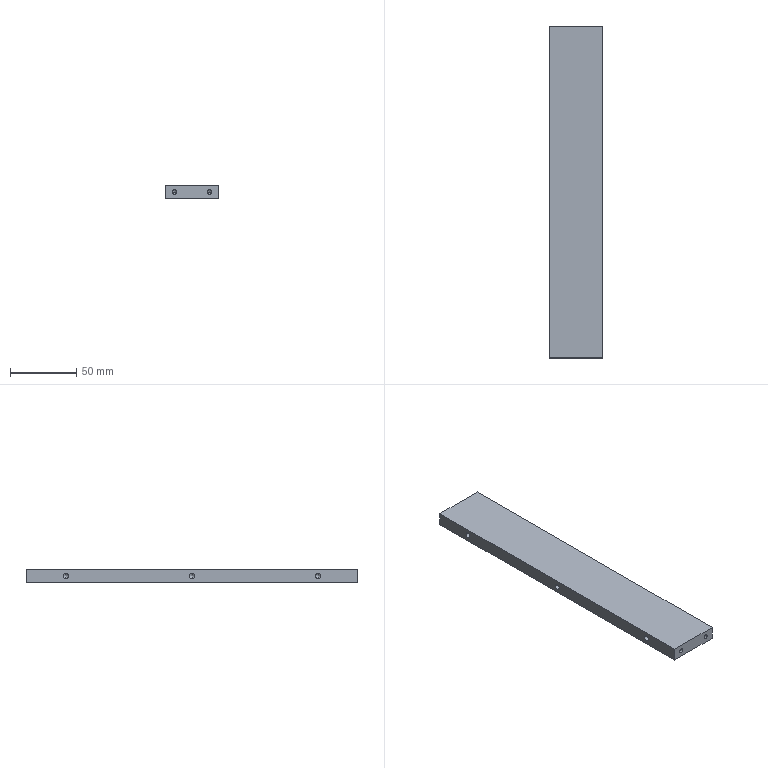Part | SolidWorks | features BaseBody 1 | 1 solid | 34 faces | box 40 x 250 x 10 mm | volume 99178 mm3 | cylinder 14 | cone 14 | plane 6 | commonest cylinder face diameters 4.134 x6 2.487 x4 3.242 x4
STEP:
#1=CARTESIAN_POINT('',(-243.627,247.034,3.757));
#2=VERTEX_POINT('',#1);
#3=CARTESIAN_POINT('',(-243.627,247.034,6.243));
#4=VERTEX_POINT('',#3);
#5=CARTESIAN_POINT('',(-243.627,247.034,5.));
#6=DIRECTION('',(0.,1.,0.));
#7=DIRECTION('',(0.,0.,1.));
#8=AXIS2_PLACEMENT_3D('',#5,#6,#7);
#9=CIRCLE('',#8,1.243);
#10=EDGE_CURVE('',#2,#4,#9,.T.);
#11=ORIENTED_EDGE('',*,*,#10,.F.);
#12=CARTESIAN_POINT('',(-243.627,259.034,3.757));
#13=VERTEX_POINT('',#12);
#14=CARTESIAN_POINT('',(-243.627,253.034,3.757));
#15=DIRECTION('',(0.,1.,0.));
#16=VECTOR('',#15,1000.);
#17=LINE('',#14,#16);
#18=EDGE_CURVE('',#2,#13,#17,.T.);
#19=ORIENTED_EDGE('',*,*,#18,.T.);
#20=CARTESIAN_POINT('',(-243.627,259.034,6.244));
#21=VERTEX_POINT('',#20);
#22=CARTESIAN_POINT('',(-243.627,259.034,5.));
#23=DIRECTION('',(0.,-1.,0.));
#24=DIRECTION('',(0.,0.,1.));
#25=AXIS2_PLACEMENT_3D('',#22,#23,#24);
#26=CIRCLE('',#25,1.243);
#27=EDGE_CURVE('',#21,#13,#26,.T.);
#28=ORIENTED_EDGE('',*,*,#27,.F.);
#29=CARTESIAN_POINT('',(-243.627,253.034,6.244));
#30=DIRECTION('',(0.,1.,0.));
#31=VECTOR('',#30,1000.);
#32=LINE('',#29,#31);
#33=EDGE_CURVE('',#4,#21,#32,.T.);
#34=ORIENTED_EDGE('',*,*,#33,.F.);
#35=EDGE_LOOP('',(#11,#19,#28,#34));
#36=FACE_OUTER_BOUND('',#35,.T.);
#37=CARTESIAN_POINT('',(-243.627,253.034,5.));
#38=DIRECTION('',(0.,1.,0.));
#39=DIRECTION('',(0.,0.,1.));
#40=AXIS2_PLACEMENT_3D('',#37,#38,#39);
#41=CYLINDRICAL_SURFACE('',#40,1.243);
#42=ADVANCED_FACE('',(#36),#41,.F.);
#43=CARTESIAN_POINT('',(-217.627,247.034,3.757));
#44=VERTEX_POINT('',#43);
#45=CARTESIAN_POINT('',(-217.627,247.034,6.243));
#46=VERTEX_POINT('',#45);
#47=CARTESIAN_POINT('',(-217.627,247.034,5.));
#48=DIRECTION('',(0.,1.,0.));
#49=DIRECTION('',(0.,0.,1.));
#50=AXIS2_PLACEMENT_3D('',#47,#48,#49);
#51=CIRCLE('',#50,1.243);
#52=EDGE_CURVE('',#44,#46,#51,.T.);
#53=ORIENTED_EDGE('',*,*,#52,.F.);
#54=CARTESIAN_POINT('',(-217.627,259.034,3.757));
#55=VERTEX_POINT('',#54);
#56=CARTESIAN_POINT('',(-217.627,253.034,3.757));
#57=DIRECTION('',(0.,1.,0.));
#58=VECTOR('',#57,1000.);
#59=LINE('',#56,#58);
#60=EDGE_CURVE('',#44,#55,#59,.T.);
#61=ORIENTED_EDGE('',*,*,#60,.T.);
#62=CARTESIAN_POINT('',(-217.627,259.034,6.244));
#63=VERTEX_POINT('',#62);
#64=CARTESIAN_POINT('',(-217.627,259.034,5.));
#65=DIRECTION('',(0.,-1.,0.));
#66=DIRECTION('',(0.,0.,1.));
#67=AXIS2_PLACEMENT_3D('',#64,#65,#66);
#68=CIRCLE('',#67,1.243);
#69=EDGE_CURVE('',#63,#55,#68,.T.);
#70=ORIENTED_EDGE('',*,*,#69,.F.);
#71=CARTESIAN_POINT('',(-217.627,253.034,6.244));
#72=DIRECTION('',(0.,1.,0.));
#73=VECTOR('',#72,1000.);
#74=LINE('',#71,#73);
#75=EDGE_CURVE('',#46,#63,#74,.T.);
#76=ORIENTED_EDGE('',*,*,#75,.F.);
#77=EDGE_LOOP('',(#53,#61,#70,#76));
#78=FACE_OUTER_BOUND('',#77,.T.);
#79=CARTESIAN_POINT('',(-217.627,253.034,5.));
#80=DIRECTION('',(0.,1.,0.));
#81=DIRECTION('',(0.,0.,1.));
#82=AXIS2_PLACEMENT_3D('',#79,#80,#81);
#83=CYLINDRICAL_SURFACE('',#82,1.243);
#84=ADVANCED_FACE('',(#78),#83,.F.);
#85=CARTESIAN_POINT('',(-245.248,21.034,5.));
#86=VERTEX_POINT('',#85);
#87=CARTESIAN_POINT('',(-242.006,21.034,5.));
#88=VERTEX_POINT('',#87);
#89=CARTESIAN_POINT('',(-243.627,21.034,5.));
#90=DIRECTION('',(0.,-1.,0.));
#91=DIRECTION('',(1.,0.,0.));
#92=AXIS2_PLACEMENT_3D('',#89,#90,#91);
#93=CIRCLE('',#92,1.621);
#94=EDGE_CURVE('',#86,#88,#93,.T.);
#95=ORIENTED_EDGE('',*,*,#94,.F.);
#96=CARTESIAN_POINT('',(-245.248,9.034,5.));
#97=VERTEX_POINT('',#96);
#98=CARTESIAN_POINT('',(-245.248,15.034,5.));
#99=DIRECTION('',(0.,-1.,0.));
#100=VECTOR('',#99,1000.);
#101=LINE('',#98,#100);
#102=EDGE_CURVE('',#86,#97,#101,.T.);
#103=ORIENTED_EDGE('',*,*,#102,.T.);
#104=CARTESIAN_POINT('',(-242.006,9.034,5.));
#105=VERTEX_POINT('',#104);
#106=CARTESIAN_POINT('',(-243.627,9.034,5.));
#107=DIRECTION('',(0.,1.,0.));
#108=DIRECTION('',(1.,0.,0.));
#109=AXIS2_PLACEMENT_3D('',#106,#107,#108);
#110=CIRCLE('',#109,1.621);
#111=EDGE_CURVE('',#105,#97,#110,.T.);
#112=ORIENTED_EDGE('',*,*,#111,.F.);
#113=CARTESIAN_POINT('',(-242.006,15.034,5.));
#114=DIRECTION('',(0.,-1.,0.));
#115=VECTOR('',#114,1000.);
#116=LINE('',#113,#115);
#117=EDGE_CURVE('',#88,#105,#116,.T.);
#118=ORIENTED_EDGE('',*,*,#117,.F.);
#119=EDGE_LOOP('',(#95,#103,#112,#118));
#120=FACE_OUTER_BOUND('',#119,.T.);
#121=CARTESIAN_POINT('',(-243.627,15.034,5.));
#122=DIRECTION('',(0.,-1.,0.));
#123=DIRECTION('',(1.,0.,0.));
#124=AXIS2_PLACEMENT_3D('',#121,#122,#123);
#125=CYLINDRICAL_SURFACE('',#124,1.621);
#126=ADVANCED_FACE('',(#120),#125,.F.);
#127=CARTESIAN_POINT('',(-219.248,21.034,5.));
#128=VERTEX_POINT('',#127);
#129=CARTESIAN_POINT('',(-216.006,21.034,5.));
#130=VERTEX_POINT('',#129);
#131=CARTESIAN_POINT('',(-217.627,21.034,5.));
#132=DIRECTION('',(0.,-1.,0.));
#133=DIRECTION('',(1.,0.,0.));
#134=AXIS2_PLACEMENT_3D('',#131,#132,#133);
#135=CIRCLE('',#134,1.621);
#136=EDGE_CURVE('',#128,#130,#135,.T.);
#137=ORIENTED_EDGE('',*,*,#136,.F.);
#138=CARTESIAN_POINT('',(-219.248,9.034,5.));
#139=VERTEX_POINT('',#138);
#140=CARTESIAN_POINT('',(-219.248,15.034,5.));
#141=DIRECTION('',(0.,-1.,0.));
#142=VECTOR('',#141,1000.);
#143=LINE('',#140,#142);
#144=EDGE_CURVE('',#128,#139,#143,.T.);
#145=ORIENTED_EDGE('',*,*,#144,.T.);
#146=CARTESIAN_POINT('',(-216.006,9.034,5.));
#147=VERTEX_POINT('',#146);
#148=CARTESIAN_POINT('',(-217.627,9.034,5.));
#149=DIRECTION('',(0.,1.,0.));
#150=DIRECTION('',(1.,0.,0.));
#151=AXIS2_PLACEMENT_3D('',#148,#149,#150);
#152=CIRCLE('',#151,1.621);
#153=EDGE_CURVE('',#147,#139,#152,.T.);
#154=ORIENTED_EDGE('',*,*,#153,.F.);
#155=CARTESIAN_POINT('',(-216.006,15.034,5.));
#156=DIRECTION('',(0.,-1.,0.));
#157=VECTOR('',#156,1000.);
#158=LINE('',#155,#157);
#159=EDGE_CURVE('',#130,#147,#158,.T.);
#160=ORIENTED_EDGE('',*,*,#159,.F.);
#161=EDGE_LOOP('',(#137,#145,#154,#160));
#162=FACE_OUTER_BOUND('',#161,.T.);
#163=CARTESIAN_POINT('',(-217.627,15.034,5.));
#164=DIRECTION('',(0.,-1.,0.));
#165=DIRECTION('',(1.,0.,0.));
#166=AXIS2_PLACEMENT_3D('',#163,#164,#165);
#167=CYLINDRICAL_SURFACE('',#166,1.621);
#168=ADVANCED_FACE('',(#162),#167,.F.);
#169=CARTESIAN_POINT('',(-238.627,231.101,5.));
#170=VERTEX_POINT('',#169);
#171=CARTESIAN_POINT('',(-238.627,229.034,2.933));
#172=VERTEX_POINT('',#171);
#173=CARTESIAN_POINT('',(-238.627,229.034,5.));
#174=DIRECTION('',(-1.,0.,0.));
#175=DIRECTION('',(0.,-1.,0.));
#176=AXIS2_PLACEMENT_3D('',#173,#174,#175);
#177=CIRCLE('',#176,2.067);
#178=EDGE_CURVE('',#170,#172,#177,.T.);
#179=ORIENTED_EDGE('',*,*,#178,.F.);
#180=CARTESIAN_POINT('',(-250.627,231.101,5.));
#181=VERTEX_POINT('',#180);
#182=CARTESIAN_POINT('',(-244.627,231.101,5.));
#183=DIRECTION('',(-1.,0.,0.));
#184=VECTOR('',#183,1000.);
#185=LINE('',#182,#184);
#186=EDGE_CURVE('',#170,#181,#185,.T.);
#187=ORIENTED_EDGE('',*,*,#186,.T.);
#188=CARTESIAN_POINT('',(-250.627,226.967,5.));
#189=VERTEX_POINT('',#188);
#190=CARTESIAN_POINT('',(-250.627,229.034,5.));
#191=DIRECTION('',(1.,0.,0.));
#192=DIRECTION('',(0.,-1.,0.));
#193=AXIS2_PLACEMENT_3D('',#190,#191,#192);
#194=CIRCLE('',#193,2.067);
#195=EDGE_CURVE('',#189,#181,#194,.T.);
#196=ORIENTED_EDGE('',*,*,#195,.F.);
#197=CARTESIAN_POINT('',(-238.627,226.967,5.));
#198=VERTEX_POINT('',#197);
#199=CARTESIAN_POINT('',(-244.627,226.967,5.));
#200=DIRECTION('',(-1.,0.,0.));
#201=VECTOR('',#200,1000.);
#202=LINE('',#199,#201);
#203=EDGE_CURVE('',#198,#189,#202,.T.);
#204=ORIENTED_EDGE('',*,*,#203,.F.);
#205=CARTESIAN_POINT('',(-238.627,229.034,5.));
#206=DIRECTION('',(-1.,0.,0.));
#207=DIRECTION('',(0.,-1.,0.));
#208=AXIS2_PLACEMENT_3D('',#205,#206,#207);
#209=CIRCLE('',#208,2.067);
#210=EDGE_CURVE('',#172,#198,#209,.T.);
#211=ORIENTED_EDGE('',*,*,#210,.F.);
#212=EDGE_LOOP('',(#179,#187,#196,#204,#211));
#213=FACE_OUTER_BOUND('',#212,.T.);
#214=CARTESIAN_POINT('',(-244.627,229.034,5.));
#215=DIRECTION('',(-1.,0.,0.));
#216=DIRECTION('',(0.,-1.,0.));
#217=AXIS2_PLACEMENT_3D('',#214,#215,#216);
#218=CYLINDRICAL_SURFACE('',#217,2.067);
#219=ADVANCED_FACE('',(#213),#218,.F.);
#220=CARTESIAN_POINT('',(-238.627,136.101,5.));
#221=VERTEX_POINT('',#220);
#222=CARTESIAN_POINT('',(-238.627,134.034,2.933));
#223=VERTEX_POINT('',#222);
#224=CARTESIAN_POINT('',(-238.627,134.034,5.));
#225=DIRECTION('',(-1.,0.,0.));
#226=DIRECTION('',(0.,-1.,0.));
#227=AXIS2_PLACEMENT_3D('',#224,#225,#226);
#228=CIRCLE('',#227,2.067);
#229=EDGE_CURVE('',#221,#223,#228,.T.);
#230=ORIENTED_EDGE('',*,*,#229,.F.);
#231=CARTESIAN_POINT('',(-250.627,136.101,5.));
#232=VERTEX_POINT('',#231);
#233=CARTESIAN_POINT('',(-244.627,136.101,5.));
#234=DIRECTION('',(-1.,0.,0.));
#235=VECTOR('',#234,1000.);
#236=LINE('',#233,#235);
#237=EDGE_CURVE('',#221,#232,#236,.T.);
#238=ORIENTED_EDGE('',*,*,#237,.T.);
#239=CARTESIAN_POINT('',(-250.627,131.967,5.));
#240=VERTEX_POINT('',#239);
#241=CARTESIAN_POINT('',(-250.627,134.034,5.));
#242=DIRECTION('',(1.,0.,0.));
#243=DIRECTION('',(0.,-1.,0.));
#244=AXIS2_PLACEMENT_3D('',#241,#242,#243);
#245=CIRCLE('',#244,2.067);
#246=EDGE_CURVE('',#240,#232,#245,.T.);
#247=ORIENTED_EDGE('',*,*,#246,.F.);
#248=CARTESIAN_POINT('',(-238.627,131.967,5.));
#249=VERTEX_POINT('',#248);
#250=CARTESIAN_POINT('',(-244.627,131.967,5.));
#251=DIRECTION('',(-1.,0.,0.));
#252=VECTOR('',#251,1000.);
#253=LINE('',#250,#252);
#254=EDGE_CURVE('',#249,#240,#253,.T.);
#255=ORIENTED_EDGE('',*,*,#254,.F.);
#256=CARTESIAN_POINT('',(-238.627,134.034,5.));
#257=DIRECTION('',(-1.,0.,0.));
#258=DIRECTION('',(0.,-1.,0.));
#259=AXIS2_PLACEMENT_3D('',#256,#257,#258);
#260=CIRCLE('',#259,2.067);
#261=EDGE_CURVE('',#223,#249,#260,.T.);
#262=ORIENTED_EDGE('',*,*,#261,.F.);
#263=EDGE_LOOP('',(#230,#238,#247,#255,#262));
#264=FACE_OUTER_BOUND('',#263,.T.);
#265=CARTESIAN_POINT('',(-244.627,134.034,5.));
#266=DIRECTION('',(-1.,0.,0.));
#267=DIRECTION('',(0.,-1.,0.));
#268=AXIS2_PLACEMENT_3D('',#265,#266,#267);
#269=CYLINDRICAL_SURFACE('',#268,2.067);
#270=ADVANCED_FACE('',(#264),#269,.F.);
#271=CARTESIAN_POINT('',(-238.627,41.101,5.));
#272=VERTEX_POINT('',#271);
#273=CARTESIAN_POINT('',(-238.627,39.034,2.933));
#274=VERTEX_POINT('',#273);
#275=CARTESIAN_POINT('',(-238.627,39.034,5.));
#276=DIRECTION('',(-1.,0.,0.));
#277=DIRECTION('',(0.,-1.,0.));
#278=AXIS2_PLACEMENT_3D('',#275,#276,#277);
#279=CIRCLE('',#278,2.067);
#280=EDGE_CURVE('',#272,#274,#279,.T.);
#281=ORIENTED_EDGE('',*,*,#280,.F.);
#282=CARTESIAN_POINT('',(-250.627,41.101,5.));
#283=VERTEX_POINT('',#282);
#284=CARTESIAN_POINT('',(-244.627,41.101,5.));
#285=DIRECTION('',(-1.,0.,0.));
#286=VECTOR('',#285,1000.);
#287=LINE('',#284,#286);
#288=EDGE_CURVE('',#272,#283,#287,.T.);
#289=ORIENTED_EDGE('',*,*,#288,.T.);
#290=CARTESIAN_POINT('',(-250.627,36.967,5.));
#291=VERTEX_POINT('',#290);
#292=CARTESIAN_POINT('',(-250.627,39.034,5.));
#293=DIRECTION('',(1.,0.,0.));
#294=DIRECTION('',(0.,-1.,0.));
#295=AXIS2_PLACEMENT_3D('',#292,#293,#294);
#296=CIRCLE('',#295,2.067);
#297=EDGE_CURVE('',#291,#283,#296,.T.);
#298=ORIENTED_EDGE('',*,*,#297,.F.);
#299=CARTESIAN_POINT('',(-238.627,36.967,5.));
#300=VERTEX_POINT('',#299);
#301=CARTESIAN_POINT('',(-244.627,36.967,5.));
#302=DIRECTION('',(-1.,0.,0.));
#303=VECTOR('',#302,1000.);
#304=LINE('',#301,#303);
#305=EDGE_CURVE('',#300,#291,#304,.T.);
#306=ORIENTED_EDGE('',*,*,#305,.F.);
#307=CARTESIAN_POINT('',(-238.627,39.034,5.));
#308=DIRECTION('',(-1.,0.,0.));
#309=DIRECTION('',(0.,-1.,0.));
#310=AXIS2_PLACEMENT_3D('',#307,#308,#309);
#311=CIRCLE('',#310,2.067);
#312=EDGE_CURVE('',#274,#300,#311,.T.);
#313=ORIENTED_EDGE('',*,*,#312,.F.);
#314=EDGE_LOOP('',(#281,#289,#298,#306,#313));
#315=FACE_OUTER_BOUND('',#314,.T.);
#316=CARTESIAN_POINT('',(-244.627,39.034,5.));
#317=DIRECTION('',(-1.,0.,0.));
#318=DIRECTION('',(0.,-1.,0.));
#319=AXIS2_PLACEMENT_3D('',#316,#317,#318);
#320=CYLINDRICAL_SURFACE('',#319,2.067);
#321=ADVANCED_FACE('',(#315),#320,.F.);
#322=CARTESIAN_POINT('',(-243.627,246.287,5.));
#323=VERTEX_POINT('',#322);
#324=CARTESIAN_POINT('',(-243.627,247.034,6.243));
#325=DIRECTION('',(0.,0.515,0.8572));
#326=VECTOR('',#325,1000.);
#327=LINE('',#324,#326);
#328=EDGE_CURVE('',#323,#4,#327,.T.);
#329=ORIENTED_EDGE('',*,*,#328,.F.);
#330=CARTESIAN_POINT('',(-243.627,247.034,3.757));
#331=DIRECTION('',(0.,0.515,-0.8572));
#332=VECTOR('',#331,1000.);
#333=LINE('',#330,#332);
#334=EDGE_CURVE('',#323,#2,#333,.T.);
#335=ORIENTED_EDGE('',*,*,#334,.T.);
#336=ORIENTED_EDGE('',*,*,#10,.T.);
#337=EDGE_LOOP('',(#329,#335,#336));
#338=FACE_OUTER_BOUND('',#337,.T.);
#339=CARTESIAN_POINT('',(-243.627,247.034,5.));
#340=DIRECTION('',(0.,1.,0.));
#341=DIRECTION('',(0.,0.,1.));
#342=AXIS2_PLACEMENT_3D('',#339,#340,#341);
#343=CONICAL_SURFACE('',#342,1.243,1.03);
#344=ADVANCED_FACE('',(#338),#343,.F.);
#345=CARTESIAN_POINT('',(-217.627,246.287,5.));
#346=VERTEX_POINT('',#345);
#347=CARTESIAN_POINT('',(-217.627,247.034,6.243));
#348=DIRECTION('',(0.,0.515,0.8572));
#349=VECTOR('',#348,1000.);
#350=LINE('',#347,#349);
#351=EDGE_CURVE('',#346,#46,#350,.T.);
#352=ORIENTED_EDGE('',*,*,#351,.F.);
#353=CARTESIAN_POINT('',(-217.627,247.034,3.757));
#354=DIRECTION('',(0.,0.515,-0.8572));
#355=VECTOR('',#354,1000.);
#356=LINE('',#353,#355);
#357=EDGE_CURVE('',#346,#44,#356,.T.);
#358=ORIENTED_EDGE('',*,*,#357,.T.);
#359=ORIENTED_EDGE('',*,*,#52,.T.);
#360=EDGE_LOOP('',(#352,#358,#359));
#361=FACE_OUTER_BOUND('',#360,.T.);
#362=CARTESIAN_POINT('',(-217.627,247.034,5.));
#363=DIRECTION('',(0.,1.,0.));
#364=DIRECTION('',(0.,0.,1.));
#365=AXIS2_PLACEMENT_3D('',#362,#363,#364);
#366=CONICAL_SURFACE('',#365,1.243,1.03);
#367=ADVANCED_FACE('',(#361),#366,.F.);
#368=CARTESIAN_POINT('',(-243.627,22.008,5.));
#369=VERTEX_POINT('',#368);
#370=CARTESIAN_POINT('',(-242.006,21.034,5.));
#371=DIRECTION('',(0.8572,-0.515,0.));
#372=VECTOR('',#371,1000.);
#373=LINE('',#370,#372);
#374=EDGE_CURVE('',#369,#88,#373,.T.);
#375=ORIENTED_EDGE('',*,*,#374,.F.);
#376=CARTESIAN_POINT('',(-245.248,21.034,5.));
#377=DIRECTION('',(-0.8572,-0.515,0.));
#378=VECTOR('',#377,1000.);
#379=LINE('',#376,#378);
#380=EDGE_CURVE('',#369,#86,#379,.T.);
#381=ORIENTED_EDGE('',*,*,#380,.T.);
#382=ORIENTED_EDGE('',*,*,#94,.T.);
#383=EDGE_LOOP('',(#375,#381,#382));
#384=FACE_OUTER_BOUND('',#383,.T.);
#385=CARTESIAN_POINT('',(-243.627,21.034,5.));
#386=DIRECTION('',(0.,-1.,0.));
#387=DIRECTION('',(1.,0.,0.));
#388=AXIS2_PLACEMENT_3D('',#385,#386,#387);
#389=CONICAL_SURFACE('',#388,1.621,1.03);
#390=ADVANCED_FACE('',(#384),#389,.F.);
#391=CARTESIAN_POINT('',(-217.627,22.008,5.));
#392=VERTEX_POINT('',#391);
#393=CARTESIAN_POINT('',(-216.006,21.034,5.));
#394=DIRECTION('',(0.8572,-0.515,0.));
#395=VECTOR('',#394,1000.);
#396=LINE('',#393,#395);
#397=EDGE_CURVE('',#392,#130,#396,.T.);
#398=ORIENTED_EDGE('',*,*,#397,.F.);
#399=CARTESIAN_POINT('',(-219.248,21.034,5.));
#400=DIRECTION('',(-0.8572,-0.515,0.));
#401=VECTOR('',#400,1000.);
#402=LINE('',#399,#401);
#403=EDGE_CURVE('',#392,#128,#402,.T.);
#404=ORIENTED_EDGE('',*,*,#403,.T.);
#405=ORIENTED_EDGE('',*,*,#136,.T.);
#406=EDGE_LOOP('',(#398,#404,#405));
#407=FACE_OUTER_BOUND('',#406,.T.);
#408=CARTESIAN_POINT('',(-217.627,21.034,5.));
#409=DIRECTION('',(0.,-1.,0.));
#410=DIRECTION('',(1.,0.,0.));
#411=AXIS2_PLACEMENT_3D('',#408,#409,#410);
#412=CONICAL_SURFACE('',#411,1.621,1.03);
#413=ADVANCED_FACE('',(#407),#412,.F.);
#414=CARTESIAN_POINT('',(-237.385,229.034,5.));
#415=VERTEX_POINT('',#414);
#416=CARTESIAN_POINT('',(-238.627,229.034,7.067));
#417=VERTEX_POINT('',#416);
#418=CARTESIAN_POINT('',(-238.627,229.034,7.067));
#419=DIRECTION('',(-0.515,0.,0.8572));
#420=VECTOR('',#419,1000.);
#421=LINE('',#418,#420);
#422=EDGE_CURVE('',#415,#417,#421,.T.);
#423=ORIENTED_EDGE('',*,*,#422,.F.);
#424=CARTESIAN_POINT('',(-238.627,229.034,2.933));
#425=DIRECTION('',(-0.515,0.,-0.8572));
#426=VECTOR('',#425,1000.);
#427=LINE('',#424,#426);
#428=EDGE_CURVE('',#415,#172,#427,.T.);
#429=ORIENTED_EDGE('',*,*,#428,.T.);
#430=ORIENTED_EDGE('',*,*,#210,.T.);
#431=CARTESIAN_POINT('',(-238.627,229.034,5.));
#432=DIRECTION('',(-1.,0.,0.));
#433=DIRECTION('',(0.,-1.,0.));
#434=AXIS2_PLACEMENT_3D('',#431,#432,#433);
#435=CIRCLE('',#434,2.067);
#436=EDGE_CURVE('',#198,#417,#435,.T.);
#437=ORIENTED_EDGE('',*,*,#436,.T.);
#438=EDGE_LOOP('',(#423,#429,#430,#437));
#439=FACE_OUTER_BOUND('',#438,.T.);
#440=CARTESIAN_POINT('',(-238.627,229.034,5.));
#441=DIRECTION('',(-1.,0.,0.));
#442=DIRECTION('',(0.,0.,1.));
#443=AXIS2_PLACEMENT_3D('',#440,#441,#442);
#444=CONICAL_SURFACE('',#443,2.067,1.03);
#445=ADVANCED_FACE('',(#439),#444,.F.);
#446=CARTESIAN_POINT('',(-237.385,134.034,5.));
#447=VERTEX_POINT('',#446);
#448=CARTESIAN_POINT('',(-238.627,134.034,7.067));
#449=VERTEX_POINT('',#448);
#450=CARTESIAN_POINT('',(-238.627,134.034,7.067));
#451=DIRECTION('',(-0.515,0.,0.8572));
#452=VECTOR('',#451,1000.);
#453=LINE('',#450,#452);
#454=EDGE_CURVE('',#447,#449,#453,.T.);
#455=ORIENTED_EDGE('',*,*,#454,.F.);
#456=CARTESIAN_POINT('',(-238.627,134.034,2.933));
#457=DIRECTION('',(-0.515,0.,-0.8572));
#458=VECTOR('',#457,1000.);
#459=LINE('',#456,#458);
#460=EDGE_CURVE('',#447,#223,#459,.T.);
#461=ORIENTED_EDGE('',*,*,#460,.T.);
#462=ORIENTED_EDGE('',*,*,#261,.T.);
#463=CARTESIAN_POINT('',(-238.627,134.034,5.));
#464=DIRECTION('',(-1.,0.,0.));
#465=DIRECTION('',(0.,-1.,0.));
#466=AXIS2_PLACEMENT_3D('',#463,#464,#465);
#467=CIRCLE('',#466,2.067);
#468=EDGE_CURVE('',#249,#449,#467,.T.);
#469=ORIENTED_EDGE('',*,*,#468,.T.);
#470=EDGE_LOOP('',(#455,#461,#462,#469));
#471=FACE_OUTER_BOUND('',#470,.T.);
#472=CARTESIAN_POINT('',(-238.627,134.034,5.));
#473=DIRECTION('',(-1.,0.,0.));
#474=DIRECTION('',(0.,0.,1.));
#475=AXIS2_PLACEMENT_3D('',#472,#473,#474);
#476=CONICAL_SURFACE('',#475,2.067,1.03);
#477=ADVANCED_FACE('',(#471),#476,.F.);
#478=CARTESIAN_POINT('',(-237.385,39.034,5.));
#479=VERTEX_POINT('',#478);
#480=CARTESIAN_POINT('',(-238.627,39.034,7.067));
#481=VERTEX_POINT('',#480);
#482=CARTESIAN_POINT('',(-238.627,39.034,7.067));
#483=DIRECTION('',(-0.515,0.,0.8572));
#484=VECTOR('',#483,1000.);
#485=LINE('',#482,#484);
#486=EDGE_CURVE('',#479,#481,#485,.T.);
#487=ORIENTED_EDGE('',*,*,#486,.F.);
#488=CARTESIAN_POINT('',(-238.627,39.034,2.933));
#489=DIRECTION('',(-0.515,0.,-0.8572));
#490=VECTOR('',#489,1000.);
#491=LINE('',#488,#490);
#492=EDGE_CURVE('',#479,#274,#491,.T.);
#493=ORIENTED_EDGE('',*,*,#492,.T.);
#494=ORIENTED_EDGE('',*,*,#312,.T.);
#495=CARTESIAN_POINT('',(-238.627,39.034,5.));
#496=DIRECTION('',(-1.,0.,0.));
#497=DIRECTION('',(0.,-1.,0.));
#498=AXIS2_PLACEMENT_3D('',#495,#496,#497);
#499=CIRCLE('',#498,2.067);
#500=EDGE_CURVE('',#300,#481,#499,.T.);
#501=ORIENTED_EDGE('',*,*,#500,.T.);
#502=EDGE_LOOP('',(#487,#493,#494,#501));
#503=FACE_OUTER_BOUND('',#502,.T.);
#504=CARTESIAN_POINT('',(-238.627,39.034,5.));
#505=DIRECTION('',(-1.,0.,0.));
#506=DIRECTION('',(0.,0.,1.));
#507=AXIS2_PLACEMENT_3D('',#504,#505,#506);
#508=CONICAL_SURFACE('',#507,2.067,1.03);
#509=ADVANCED_FACE('',(#503),#508,.F.);
#510=CARTESIAN_POINT('',(-210.627,9.034,0.));
#511=VERTEX_POINT('',#510);
#512=CARTESIAN_POINT('',(-210.627,259.034,0.));
#513=VERTEX_POINT('',#512);
#514=CARTESIAN_POINT('',(-210.627,134.034,0.));
#515=DIRECTION('',(0.,1.,0.));
#516=VECTOR('',#515,1000.);
#517=LINE('',#514,#516);
#518=EDGE_CURVE('',#511,#513,#517,.T.);
#519=ORIENTED_EDGE('',*,*,#518,.F.);
#520=CARTESIAN_POINT('',(-250.627,9.034,0.));
#521=VERTEX_POINT('',#520);
#522=CARTESIAN_POINT('',(-230.627,9.034,0.));
#523=DIRECTION('',(1.,0.,0.));
#524=VECTOR('',#523,1000.);
#525=LINE('',#522,#524);
#526=EDGE_CURVE('',#521,#511,#525,.T.);
#527=ORIENTED_EDGE('',*,*,#526,.F.);
#528=CARTESIAN_POINT('',(-250.627,259.034,0.));
#529=VERTEX_POINT('',#528);
#530=CARTESIAN_POINT('',(-250.627,134.034,0.));
#531=DIRECTION('',(0.,-1.,0.));
#532=VECTOR('',#531,1000.);
#533=LINE('',#530,#532);
#534=EDGE_CURVE('',#529,#521,#533,.T.);
#535=ORIENTED_EDGE('',*,*,#534,.F.);
#536=CARTESIAN_POINT('',(-230.627,259.034,0.));
#537=DIRECTION('',(-1.,0.,0.));
#538=VECTOR('',#537,1000.);
#539=LINE('',#536,#538);
#540=EDGE_CURVE('',#513,#529,#539,.T.);
#541=ORIENTED_EDGE('',*,*,#540,.F.);
#542=EDGE_LOOP('',(#519,#527,#535,#541));
#543=FACE_OUTER_BOUND('',#542,.T.);
#544=CARTESIAN_POINT('',(-230.627,134.034,0.));
#545=DIRECTION('',(0.,0.,1.));
#546=DIRECTION('',(1.,0.,0.));
#547=AXIS2_PLACEMENT_3D('',#544,#545,#546);
#548=PLANE('',#547);
#549=ADVANCED_FACE('',(#543),#548,.F.);
#550=ORIENTED_EDGE('',*,*,#27,.T.);
#551=CARTESIAN_POINT('',(-243.627,259.034,5.));
#552=DIRECTION('',(0.,-1.,0.));
#553=DIRECTION('',(0.,0.,1.));
#554=AXIS2_PLACEMENT_3D('',#551,#552,#553);
#555=CIRCLE('',#554,1.243);
#556=EDGE_CURVE('',#13,#21,#555,.T.);
#557=ORIENTED_EDGE('',*,*,#556,.T.);
#558=EDGE_LOOP('',(#550,#557));
#559=FACE_BOUND('',#558,.T.);
#560=ORIENTED_EDGE('',*,*,#69,.T.);
#561=CARTESIAN_POINT('',(-217.627,259.034,5.));
#562=DIRECTION('',(0.,-1.,0.));
#563=DIRECTION('',(0.,0.,1.));
#564=AXIS2_PLACEMENT_3D('',#561,#562,#563);
#565=CIRCLE('',#564,1.243);
#566=EDGE_CURVE('',#55,#63,#565,.T.);
#567=ORIENTED_EDGE('',*,*,#566,.T.);
#568=EDGE_LOOP('',(#560,#567));
#569=FACE_BOUND('',#568,.T.);
#570=ORIENTED_EDGE('',*,*,#540,.T.);
#571=CARTESIAN_POINT('',(-250.627,259.034,10.));
#572=VERTEX_POINT('',#571);
#573=CARTESIAN_POINT('',(-250.627,259.034,0.));
#574=DIRECTION('',(0.,0.,1.));
#575=VECTOR('',#574,1000.);
#576=LINE('',#573,#575);
#577=EDGE_CURVE('',#529,#572,#576,.T.);
#578=ORIENTED_EDGE('',*,*,#577,.T.);
#579=CARTESIAN_POINT('',(-210.627,259.034,10.));
#580=VERTEX_POINT('',#579);
#581=CARTESIAN_POINT('',(-250.627,259.034,10.));
#582=DIRECTION('',(1.,0.,0.));
#583=VECTOR('',#582,1000.);
#584=LINE('',#581,#583);
#585=EDGE_CURVE('',#572,#580,#584,.T.);
#586=ORIENTED_EDGE('',*,*,#585,.T.);
#587=CARTESIAN_POINT('',(-210.627,259.034,0.));
#588=DIRECTION('',(0.,0.,-1.));
#589=VECTOR('',#588,1000.);
#590=LINE('',#587,#589);
#591=EDGE_CURVE('',#580,#513,#590,.T.);
#592=ORIENTED_EDGE('',*,*,#591,.T.);
#593=EDGE_LOOP('',(#570,#578,#586,#592));
#594=FACE_OUTER_BOUND('',#593,.T.);
#595=CARTESIAN_POINT('',(-250.627,259.034,0.));
#596=DIRECTION('',(0.,1.,0.));
#597=DIRECTION('',(0.,0.,1.));
#598=AXIS2_PLACEMENT_3D('',#595,#596,#597);
#599=PLANE('',#598);
#600=ADVANCED_FACE('',(#559,#569,#594),#599,.T.);
#601=ORIENTED_EDGE('',*,*,#518,.T.);
#602=ORIENTED_EDGE('',*,*,#591,.F.);
#603=CARTESIAN_POINT('',(-210.627,9.034,10.));
#604=VERTEX_POINT('',#603);
#605=CARTESIAN_POINT('',(-210.627,259.034,10.));
#606=DIRECTION('',(0.,-1.,0.));
#607=VECTOR('',#606,1000.);
#608=LINE('',#605,#607);
#609=EDGE_CURVE('',#580,#604,#608,.T.);
#610=ORIENTED_EDGE('',*,*,#609,.T.);
#611=CARTESIAN_POINT('',(-210.627,9.034,0.));
#612=DIRECTION('',(0.,0.,-1.));
#613=VECTOR('',#612,1000.);
#614=LINE('',#611,#613);
#615=EDGE_CURVE('',#604,#511,#614,.T.);
#616=ORIENTED_EDGE('',*,*,#615,.T.);
#617=EDGE_LOOP('',(#601,#602,#610,#616));
#618=FACE_OUTER_BOUND('',#617,.T.);
#619=CARTESIAN_POINT('',(-210.627,259.034,0.));
#620=DIRECTION('',(1.,0.,0.));
#621=DIRECTION('',(0.,0.,-1.));
#622=AXIS2_PLACEMENT_3D('',#619,#620,#621);
#623=PLANE('',#622);
#624=ADVANCED_FACE('',(#618),#623,.T.);
#625=ORIENTED_EDGE('',*,*,#111,.T.);
#626=CARTESIAN_POINT('',(-243.627,9.034,5.));
#627=DIRECTION('',(0.,1.,0.));
#628=DIRECTION('',(1.,0.,0.));
#629=AXIS2_PLACEMENT_3D('',#626,#627,#628);
#630=CIRCLE('',#629,1.621);
#631=EDGE_CURVE('',#97,#105,#630,.T.);
#632=ORIENTED_EDGE('',*,*,#631,.T.);
#633=EDGE_LOOP('',(#625,#632));
#634=FACE_BOUND('',#633,.T.);
#635=ORIENTED_EDGE('',*,*,#153,.T.);
#636=CARTESIAN_POINT('',(-217.627,9.034,5.));
#637=DIRECTION('',(0.,1.,0.));
#638=DIRECTION('',(1.,0.,0.));
#639=AXIS2_PLACEMENT_3D('',#636,#637,#638);
#640=CIRCLE('',#639,1.621);
#641=EDGE_CURVE('',#139,#147,#640,.T.);
#642=ORIENTED_EDGE('',*,*,#641,.T.);
#643=EDGE_LOOP('',(#635,#642));
#644=FACE_BOUND('',#643,.T.);
#645=ORIENTED_EDGE('',*,*,#526,.T.);
#646=ORIENTED_EDGE('',*,*,#615,.F.);
#647=CARTESIAN_POINT('',(-250.627,9.034,10.));
#648=VERTEX_POINT('',#647);
#649=CARTESIAN_POINT('',(-210.627,9.034,10.));
#650=DIRECTION('',(-1.,0.,0.));
#651=VECTOR('',#650,1000.);
#652=LINE('',#649,#651);
#653=EDGE_CURVE('',#604,#648,#652,.T.);
#654=ORIENTED_EDGE('',*,*,#653,.T.);
#655=CARTESIAN_POINT('',(-250.627,9.034,0.));
#656=DIRECTION('',(0.,0.,-1.));
#657=VECTOR('',#656,1000.);
#658=LINE('',#655,#657);
#659=EDGE_CURVE('',#648,#521,#658,.T.);
#660=ORIENTED_EDGE('',*,*,#659,.T.);
#661=EDGE_LOOP('',(#645,#646,#654,#660));
#662=FACE_OUTER_BOUND('',#661,.T.);
#663=CARTESIAN_POINT('',(-210.627,9.034,0.));
#664=DIRECTION('',(0.,-1.,0.));
#665=DIRECTION('',(0.,0.,-1.));
#666=AXIS2_PLACEMENT_3D('',#663,#664,#665);
#667=PLANE('',#666);
#668=ADVANCED_FACE('',(#634,#644,#662),#667,.T.);
#669=ORIENTED_EDGE('',*,*,#195,.T.);
#670=CARTESIAN_POINT('',(-250.627,229.034,5.));
#671=DIRECTION('',(1.,0.,0.));
#672=DIRECTION('',(0.,-1.,0.));
#673=AXIS2_PLACEMENT_3D('',#670,#671,#672);
#674=CIRCLE('',#673,2.067);
#675=EDGE_CURVE('',#181,#189,#674,.T.);
#676=ORIENTED_EDGE('',*,*,#675,.T.);
#677=EDGE_LOOP('',(#669,#676));
#678=FACE_BOUND('',#677,.T.);
#679=ORIENTED_EDGE('',*,*,#246,.T.);
#680=CARTESIAN_POINT('',(-250.627,134.034,5.));
#681=DIRECTION('',(1.,0.,0.));
#682=DIRECTION('',(0.,-1.,0.));
#683=AXIS2_PLACEMENT_3D('',#680,#681,#682);
#684=CIRCLE('',#683,2.067);
#685=EDGE_CURVE('',#232,#240,#684,.T.);
#686=ORIENTED_EDGE('',*,*,#685,.T.);
#687=EDGE_LOOP('',(#679,#686));
#688=FACE_BOUND('',#687,.T.);
#689=ORIENTED_EDGE('',*,*,#297,.T.);
#690=CARTESIAN_POINT('',(-250.627,39.034,5.));
#691=DIRECTION('',(1.,0.,0.));
#692=DIRECTION('',(0.,-1.,0.));
#693=AXIS2_PLACEMENT_3D('',#690,#691,#692);
#694=CIRCLE('',#693,2.067);
#695=EDGE_CURVE('',#283,#291,#694,.T.);
#696=ORIENTED_EDGE('',*,*,#695,.T.);
#697=EDGE_LOOP('',(#689,#696));
#698=FACE_BOUND('',#697,.T.);
#699=ORIENTED_EDGE('',*,*,#534,.T.);
#700=ORIENTED_EDGE('',*,*,#659,.F.);
#701=CARTESIAN_POINT('',(-250.627,9.034,10.));
#702=DIRECTION('',(0.,1.,0.));
#703=VECTOR('',#702,1000.);
#704=LINE('',#701,#703);
#705=EDGE_CURVE('',#648,#572,#704,.T.);
#706=ORIENTED_EDGE('',*,*,#705,.T.);
#707=ORIENTED_EDGE('',*,*,#577,.F.);
#708=EDGE_LOOP('',(#699,#700,#706,#707));
#709=FACE_OUTER_BOUND('',#708,.T.);
#710=CARTESIAN_POINT('',(-250.627,9.034,0.));
#711=DIRECTION('',(-1.,0.,0.));
#712=DIRECTION('',(0.,0.,1.));
#713=AXIS2_PLACEMENT_3D('',#710,#711,#712);
#714=PLANE('',#713);
#715=ADVANCED_FACE('',(#678,#688,#698,#709),#714,.T.);
#716=ORIENTED_EDGE('',*,*,#18,.F.);
#717=CARTESIAN_POINT('',(-243.627,247.034,5.));
#718=DIRECTION('',(0.,1.,0.));
#719=DIRECTION('',(0.,0.,1.));
#720=AXIS2_PLACEMENT_3D('',#717,#718,#719);
#721=CIRCLE('',#720,1.243);
#722=EDGE_CURVE('',#4,#2,#721,.T.);
#723=ORIENTED_EDGE('',*,*,#722,.F.);
#724=ORIENTED_EDGE('',*,*,#33,.T.);
#725=ORIENTED_EDGE('',*,*,#556,.F.);
#726=EDGE_LOOP('',(#716,#723,#724,#725));
#727=FACE_OUTER_BOUND('',#726,.T.);
#728=CARTESIAN_POINT('',(-243.627,253.034,5.));
#729=DIRECTION('',(0.,1.,0.));
#730=DIRECTION('',(0.,0.,1.));
#731=AXIS2_PLACEMENT_3D('',#728,#729,#730);
#732=CYLINDRICAL_SURFACE('',#731,1.243);
#733=ADVANCED_FACE('',(#727),#732,.F.);
#734=ORIENTED_EDGE('',*,*,#60,.F.);
#735=CARTESIAN_POINT('',(-217.627,247.034,5.));
#736=DIRECTION('',(0.,1.,0.));
#737=DIRECTION('',(0.,0.,1.));
#738=AXIS2_PLACEMENT_3D('',#735,#736,#737);
#739=CIRCLE('',#738,1.243);
#740=EDGE_CURVE('',#46,#44,#739,.T.);
#741=ORIENTED_EDGE('',*,*,#740,.F.);
#742=ORIENTED_EDGE('',*,*,#75,.T.);
#743=ORIENTED_EDGE('',*,*,#566,.F.);
#744=EDGE_LOOP('',(#734,#741,#742,#743));
#745=FACE_OUTER_BOUND('',#744,.T.);
#746=CARTESIAN_POINT('',(-217.627,253.034,5.));
#747=DIRECTION('',(0.,1.,0.));
#748=DIRECTION('',(0.,0.,1.));
#749=AXIS2_PLACEMENT_3D('',#746,#747,#748);
#750=CYLINDRICAL_SURFACE('',#749,1.243);
#751=ADVANCED_FACE('',(#745),#750,.F.);
#752=ORIENTED_EDGE('',*,*,#705,.F.);
#753=ORIENTED_EDGE('',*,*,#653,.F.);
#754=ORIENTED_EDGE('',*,*,#609,.F.);
#755=ORIENTED_EDGE('',*,*,#585,.F.);
#756=EDGE_LOOP('',(#752,#753,#754,#755));
#757=FACE_OUTER_BOUND('',#756,.T.);
#758=CARTESIAN_POINT('',(-230.627,134.034,10.));
#759=DIRECTION('',(0.,0.,1.));
#760=DIRECTION('',(1.,0.,0.));
#761=AXIS2_PLACEMENT_3D('',#758,#759,#760);
#762=PLANE('',#761);
#763=ADVANCED_FACE('',(#757),#762,.T.);
#764=ORIENTED_EDGE('',*,*,#102,.F.);
#765=CARTESIAN_POINT('',(-243.627,21.034,5.));
#766=DIRECTION('',(0.,-1.,0.));
#767=DIRECTION('',(1.,0.,0.));
#768=AXIS2_PLACEMENT_3D('',#765,#766,#767);
#769=CIRCLE('',#768,1.621);
#770=EDGE_CURVE('',#88,#86,#769,.T.);
#771=ORIENTED_EDGE('',*,*,#770,.F.);
#772=ORIENTED_EDGE('',*,*,#117,.T.);
#773=ORIENTED_EDGE('',*,*,#631,.F.);
#774=EDGE_LOOP('',(#764,#771,#772,#773));
#775=FACE_OUTER_BOUND('',#774,.T.);
#776=CARTESIAN_POINT('',(-243.627,15.034,5.));
#777=DIRECTION('',(0.,-1.,0.));
#778=DIRECTION('',(1.,0.,0.));
#779=AXIS2_PLACEMENT_3D('',#776,#777,#778);
#780=CYLINDRICAL_SURFACE('',#779,1.621);
#781=ADVANCED_FACE('',(#775),#780,.F.);
#782=ORIENTED_EDGE('',*,*,#144,.F.);
#783=CARTESIAN_POINT('',(-217.627,21.034,5.));
#784=DIRECTION('',(0.,-1.,0.));
#785=DIRECTION('',(1.,0.,0.));
#786=AXIS2_PLACEMENT_3D('',#783,#784,#785);
#787=CIRCLE('',#786,1.621);
#788=EDGE_CURVE('',#130,#128,#787,.T.);
#789=ORIENTED_EDGE('',*,*,#788,.F.);
#790=ORIENTED_EDGE('',*,*,#159,.T.);
#791=ORIENTED_EDGE('',*,*,#641,.F.);
#792=EDGE_LOOP('',(#782,#789,#790,#791));
#793=FACE_OUTER_BOUND('',#792,.T.);
#794=CARTESIAN_POINT('',(-217.627,15.034,5.));
#795=DIRECTION('',(0.,-1.,0.));
#796=DIRECTION('',(1.,0.,0.));
#797=AXIS2_PLACEMENT_3D('',#794,#795,#796);
#798=CYLINDRICAL_SURFACE('',#797,1.621);
#799=ADVANCED_FACE('',(#793),#798,.F.);
#800=ORIENTED_EDGE('',*,*,#186,.F.);
#801=CARTESIAN_POINT('',(-238.627,229.034,5.));
#802=DIRECTION('',(-1.,0.,0.));
#803=DIRECTION('',(0.,-1.,0.));
#804=AXIS2_PLACEMENT_3D('',#801,#802,#803);
#805=CIRCLE('',#804,2.067);
#806=EDGE_CURVE('',#417,#170,#805,.T.);
#807=ORIENTED_EDGE('',*,*,#806,.F.);
#808=ORIENTED_EDGE('',*,*,#436,.F.);
#809=ORIENTED_EDGE('',*,*,#203,.T.);
#810=ORIENTED_EDGE('',*,*,#675,.F.);
#811=EDGE_LOOP('',(#800,#807,#808,#809,#810));
#812=FACE_OUTER_BOUND('',#811,.T.);
#813=CARTESIAN_POINT('',(-244.627,229.034,5.));
#814=DIRECTION('',(-1.,0.,0.));
#815=DIRECTION('',(0.,-1.,0.));
#816=AXIS2_PLACEMENT_3D('',#813,#814,#815);
#817=CYLINDRICAL_SURFACE('',#816,2.067);
#818=ADVANCED_FACE('',(#812),#817,.F.);
#819=ORIENTED_EDGE('',*,*,#237,.F.);
#820=CARTESIAN_POINT('',(-238.627,134.034,5.));
#821=DIRECTION('',(-1.,0.,0.));
#822=DIRECTION('',(0.,-1.,0.));
#823=AXIS2_PLACEMENT_3D('',#820,#821,#822);
#824=CIRCLE('',#823,2.067);
#825=EDGE_CURVE('',#449,#221,#824,.T.);
#826=ORIENTED_EDGE('',*,*,#825,.F.);
#827=ORIENTED_EDGE('',*,*,#468,.F.);
#828=ORIENTED_EDGE('',*,*,#254,.T.);
#829=ORIENTED_EDGE('',*,*,#685,.F.);
#830=EDGE_LOOP('',(#819,#826,#827,#828,#829));
#831=FACE_OUTER_BOUND('',#830,.T.);
#832=CARTESIAN_POINT('',(-244.627,134.034,5.));
#833=DIRECTION('',(-1.,0.,0.));
#834=DIRECTION('',(0.,-1.,0.));
#835=AXIS2_PLACEMENT_3D('',#832,#833,#834);
#836=CYLINDRICAL_SURFACE('',#835,2.067);
#837=ADVANCED_FACE('',(#831),#836,.F.);
#838=ORIENTED_EDGE('',*,*,#288,.F.);
#839=CARTESIAN_POINT('',(-238.627,39.034,5.));
#840=DIRECTION('',(-1.,0.,0.));
#841=DIRECTION('',(0.,-1.,0.));
#842=AXIS2_PLACEMENT_3D('',#839,#840,#841);
#843=CIRCLE('',#842,2.067);
#844=EDGE_CURVE('',#481,#272,#843,.T.);
#845=ORIENTED_EDGE('',*,*,#844,.F.);
#846=ORIENTED_EDGE('',*,*,#500,.F.);
#847=ORIENTED_EDGE('',*,*,#305,.T.);
#848=ORIENTED_EDGE('',*,*,#695,.F.);
#849=EDGE_LOOP('',(#838,#845,#846,#847,#848));
#850=FACE_OUTER_BOUND('',#849,.T.);
#851=CARTESIAN_POINT('',(-244.627,39.034,5.));
#852=DIRECTION('',(-1.,0.,0.));
#853=DIRECTION('',(0.,-1.,0.));
#854=AXIS2_PLACEMENT_3D('',#851,#852,#853);
#855=CYLINDRICAL_SURFACE('',#854,2.067);
#856=ADVANCED_FACE('',(#850),#855,.F.);
#857=ORIENTED_EDGE('',*,*,#334,.F.);
#858=ORIENTED_EDGE('',*,*,#328,.T.);
#859=ORIENTED_EDGE('',*,*,#722,.T.);
#860=EDGE_LOOP('',(#857,#858,#859));
#861=FACE_OUTER_BOUND('',#860,.T.);
#862=CARTESIAN_POINT('',(-243.627,247.034,5.));
#863=DIRECTION('',(0.,1.,0.));
#864=DIRECTION('',(0.,0.,1.));
#865=AXIS2_PLACEMENT_3D('',#862,#863,#864);
#866=CONICAL_SURFACE('',#865,1.243,1.03);
#867=ADVANCED_FACE('',(#861),#866,.F.);
#868=ORIENTED_EDGE('',*,*,#357,.F.);
#869=ORIENTED_EDGE('',*,*,#351,.T.);
#870=ORIENTED_EDGE('',*,*,#740,.T.);
#871=EDGE_LOOP('',(#868,#869,#870));
#872=FACE_OUTER_BOUND('',#871,.T.);
#873=CARTESIAN_POINT('',(-217.627,247.034,5.));
#874=DIRECTION('',(0.,1.,0.));
#875=DIRECTION('',(0.,0.,1.));
#876=AXIS2_PLACEMENT_3D('',#873,#874,#875);
#877=CONICAL_SURFACE('',#876,1.243,1.03);
#878=ADVANCED_FACE('',(#872),#877,.F.);
#879=ORIENTED_EDGE('',*,*,#380,.F.);
#880=ORIENTED_EDGE('',*,*,#374,.T.);
#881=ORIENTED_EDGE('',*,*,#770,.T.);
#882=EDGE_LOOP('',(#879,#880,#881));
#883=FACE_OUTER_BOUND('',#882,.T.);
#884=CARTESIAN_POINT('',(-243.627,21.034,5.));
#885=DIRECTION('',(0.,-1.,0.));
#886=DIRECTION('',(1.,0.,0.));
#887=AXIS2_PLACEMENT_3D('',#884,#885,#886);
#888=CONICAL_SURFACE('',#887,1.621,1.03);
#889=ADVANCED_FACE('',(#883),#888,.F.);
#890=ORIENTED_EDGE('',*,*,#403,.F.);
#891=ORIENTED_EDGE('',*,*,#397,.T.);
#892=ORIENTED_EDGE('',*,*,#788,.T.);
#893=EDGE_LOOP('',(#890,#891,#892));
#894=FACE_OUTER_BOUND('',#893,.T.);
#895=CARTESIAN_POINT('',(-217.627,21.034,5.));
#896=DIRECTION('',(0.,-1.,0.));
#897=DIRECTION('',(1.,0.,0.));
#898=AXIS2_PLACEMENT_3D('',#895,#896,#897);
#899=CONICAL_SURFACE('',#898,1.621,1.03);
#900=ADVANCED_FACE('',(#894),#899,.F.);
#901=ORIENTED_EDGE('',*,*,#428,.F.);
#902=ORIENTED_EDGE('',*,*,#422,.T.);
#903=ORIENTED_EDGE('',*,*,#806,.T.);
#904=ORIENTED_EDGE('',*,*,#178,.T.);
#905=EDGE_LOOP('',(#901,#902,#903,#904));
#906=FACE_OUTER_BOUND('',#905,.T.);
#907=CARTESIAN_POINT('',(-238.627,229.034,5.));
#908=DIRECTION('',(-1.,0.,0.));
#909=DIRECTION('',(0.,0.,1.));
#910=AXIS2_PLACEMENT_3D('',#907,#908,#909);
#911=CONICAL_SURFACE('',#910,2.067,1.03);
#912=ADVANCED_FACE('',(#906),#911,.F.);
#913=ORIENTED_EDGE('',*,*,#460,.F.);
#914=ORIENTED_EDGE('',*,*,#454,.T.);
#915=ORIENTED_EDGE('',*,*,#825,.T.);
#916=ORIENTED_EDGE('',*,*,#229,.T.);
#917=EDGE_LOOP('',(#913,#914,#915,#916));
#918=FACE_OUTER_BOUND('',#917,.T.);
#919=CARTESIAN_POINT('',(-238.627,134.034,5.));
#920=DIRECTION('',(-1.,0.,0.));
#921=DIRECTION('',(0.,0.,1.));
#922=AXIS2_PLACEMENT_3D('',#919,#920,#921);
#923=CONICAL_SURFACE('',#922,2.067,1.03);
#924=ADVANCED_FACE('',(#918),#923,.F.);
#925=ORIENTED_EDGE('',*,*,#492,.F.);
#926=ORIENTED_EDGE('',*,*,#486,.T.);
#927=ORIENTED_EDGE('',*,*,#844,.T.);
#928=ORIENTED_EDGE('',*,*,#280,.T.);
#929=EDGE_LOOP('',(#925,#926,#927,#928));
#930=FACE_OUTER_BOUND('',#929,.T.);
#931=CARTESIAN_POINT('',(-238.627,39.034,5.));
#932=DIRECTION('',(-1.,0.,0.));
#933=DIRECTION('',(0.,0.,1.));
#934=AXIS2_PLACEMENT_3D('',#931,#932,#933);
#935=CONICAL_SURFACE('',#934,2.067,1.03);
#936=ADVANCED_FACE('',(#930),#935,.F.);
#937=CLOSED_SHELL('',(#42,#84,#126,#168,#219,#270,#321,#344,#367,#390,#413,#445,#477,#509,#549,#600,#624,#668,#715,#733,#751,#763,#781,#799,#818,#837,#856,#867,#878,#889,#900,#912,#924,#936));
#938=MANIFOLD_SOLID_BREP('',#937);
#939=CARTESIAN_POINT('',(0.,0.,0.));
#940=DIRECTION('',(0.,0.,1.));
#941=DIRECTION('',(1.,0.,0.));
#942=AXIS2_PLACEMENT_3D('',#939,#940,#941);
#943=(LENGTH_UNIT()NAMED_UNIT(*)SI_UNIT(.MILLI.,.METRE.));
#944=UNCERTAINTY_MEASURE_WITH_UNIT(LENGTH_MEASURE(0.00001),#943,'','');
#945=(NAMED_UNIT(*)PLANE_ANGLE_UNIT()SI_UNIT($,.RADIAN.));
#946=(NAMED_UNIT(*)SI_UNIT($,.STERADIAN.)SOLID_ANGLE_UNIT());
#947=(GEOMETRIC_REPRESENTATION_CONTEXT(3)GLOBAL_UNCERTAINTY_ASSIGNED_CONTEXT((#944))GLOBAL_UNIT_ASSIGNED_CONTEXT((#943,#945,#946))REPRESENTATION_CONTEXT('',''));
#948=ADVANCED_BREP_SHAPE_REPRESENTATION('',(#938,#942),#947);